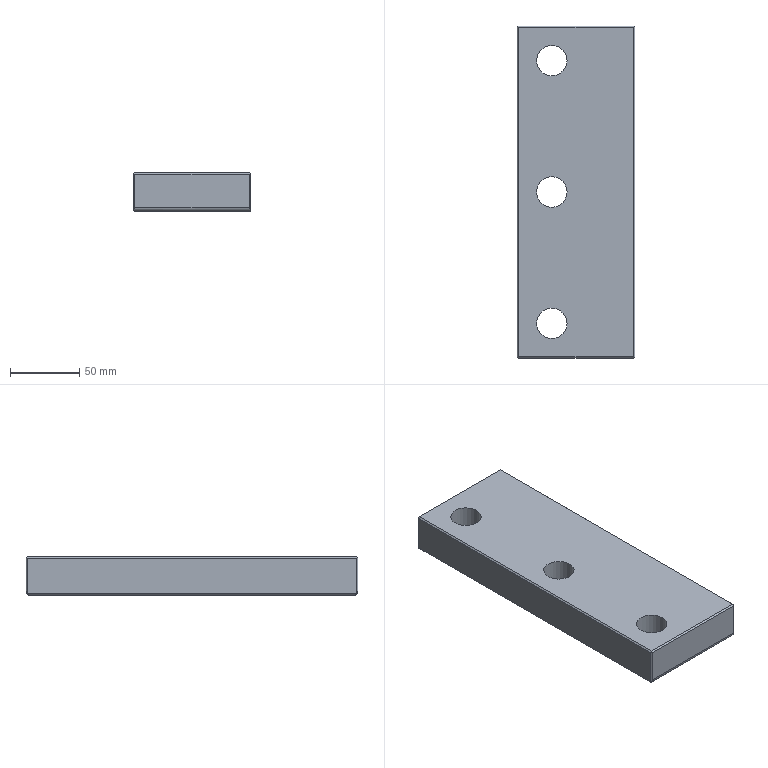Part | NX | features solid 2 | 1 solid | 21 faces | box 85 x 240 x 28 mm | volume 538397 mm3 | plane 15 | cylinder 6 | commonest cylinder face diameters 22 x3 6 x2 2 x1
STEP:
#1=CARTESIAN_POINT('',(-565.,441.,89.));
#2=VERTEX_POINT('',#1);
#3=CARTESIAN_POINT('',(-565.,441.,63.));
#4=VERTEX_POINT('',#3);
#5=CARTESIAN_POINT('',(-565.,441.,62.));
#6=DIRECTION('',(0.,0.,-1.));
#7=VECTOR('',#6,1000.);
#8=LINE('',#5,#7);
#9=EDGE_CURVE('',#2,#4,#8,.T.);
#10=ORIENTED_EDGE('',*,*,#9,.T.);
#11=CARTESIAN_POINT('',(-565.,679.,63.));
#12=VERTEX_POINT('',#11);
#13=CARTESIAN_POINT('',(-565.,680.,63.));
#14=DIRECTION('',(0.,-1.,0.));
#15=VECTOR('',#14,1000.);
#16=LINE('',#13,#15);
#17=EDGE_CURVE('',#4,#12,#16,.F.);
#18=ORIENTED_EDGE('',*,*,#17,.T.);
#19=CARTESIAN_POINT('',(-565.,679.,89.));
#20=VERTEX_POINT('',#19);
#21=CARTESIAN_POINT('',(-565.,679.,62.));
#22=DIRECTION('',(0.,0.,1.));
#23=VECTOR('',#22,1000.);
#24=LINE('',#21,#23);
#25=EDGE_CURVE('',#12,#20,#24,.T.);
#26=ORIENTED_EDGE('',*,*,#25,.T.);
#27=CARTESIAN_POINT('',(-565.,680.,89.));
#28=DIRECTION('',(0.,-1.,0.));
#29=VECTOR('',#28,1000.);
#30=LINE('',#27,#29);
#31=EDGE_CURVE('',#20,#2,#30,.T.);
#32=ORIENTED_EDGE('',*,*,#31,.T.);
#33=EDGE_LOOP('',(#10,#18,#26,#32));
#34=FACE_BOUND('',#33,.T.);
#35=CARTESIAN_POINT('',(-565.,680.,62.));
#36=DIRECTION('',(1.,0.,0.));
#37=DIRECTION('',(0.,0.,-1.));
#38=AXIS2_PLACEMENT_3D('',#35,#36,#37);
#39=PLANE('',#38);
#40=ADVANCED_FACE('',(#34),#39,.T.);
#41=CARTESIAN_POINT('',(-614.,655.,90.));
#42=VERTEX_POINT('',#41);
#43=CARTESIAN_POINT('',(-625.,655.,90.));
#44=DIRECTION('',(0.,0.,1.));
#45=DIRECTION('',(1.,0.,0.));
#46=AXIS2_PLACEMENT_3D('',#43,#44,#45);
#47=CIRCLE('',#46,11.);
#48=EDGE_CURVE('',#42,#42,#47,.T.);
#49=ORIENTED_EDGE('',*,*,#48,.F.);
#50=EDGE_LOOP('',(#49));
#51=FACE_BOUND('',#50,.T.);
#52=CARTESIAN_POINT('',(-614.,560.,90.));
#53=VERTEX_POINT('',#52);
#54=CARTESIAN_POINT('',(-625.,560.,90.));
#55=DIRECTION('',(0.,0.,1.));
#56=DIRECTION('',(1.,0.,0.));
#57=AXIS2_PLACEMENT_3D('',#54,#55,#56);
#58=CIRCLE('',#57,11.);
#59=EDGE_CURVE('',#53,#53,#58,.T.);
#60=ORIENTED_EDGE('',*,*,#59,.F.);
#61=EDGE_LOOP('',(#60));
#62=FACE_BOUND('',#61,.T.);
#63=CARTESIAN_POINT('',(-614.,465.,90.));
#64=VERTEX_POINT('',#63);
#65=CARTESIAN_POINT('',(-625.,465.,90.));
#66=DIRECTION('',(0.,0.,1.));
#67=DIRECTION('',(1.,0.,0.));
#68=AXIS2_PLACEMENT_3D('',#65,#66,#67);
#69=CIRCLE('',#68,11.);
#70=EDGE_CURVE('',#64,#64,#69,.T.);
#71=ORIENTED_EDGE('',*,*,#70,.F.);
#72=EDGE_LOOP('',(#71));
#73=FACE_BOUND('',#72,.T.);
#74=CARTESIAN_POINT('',(-649.,679.,90.));
#75=VERTEX_POINT('',#74);
#76=CARTESIAN_POINT('',(-649.,441.,90.));
#77=VERTEX_POINT('',#76);
#78=CARTESIAN_POINT('',(-649.,680.,90.));
#79=DIRECTION('',(0.,-1.,0.));
#80=VECTOR('',#79,1000.);
#81=LINE('',#78,#80);
#82=EDGE_CURVE('',#75,#77,#81,.T.);
#83=ORIENTED_EDGE('',*,*,#82,.T.);
#84=CARTESIAN_POINT('',(-566.,441.,90.));
#85=VERTEX_POINT('',#84);
#86=CARTESIAN_POINT('',(-566.,441.,90.));
#87=DIRECTION('',(1.,0.,0.));
#88=VECTOR('',#87,1000.);
#89=LINE('',#86,#88);
#90=EDGE_CURVE('',#77,#85,#89,.T.);
#91=ORIENTED_EDGE('',*,*,#90,.T.);
#92=CARTESIAN_POINT('',(-566.,679.,90.));
#93=VERTEX_POINT('',#92);
#94=CARTESIAN_POINT('',(-566.,680.,90.));
#95=DIRECTION('',(0.,1.,0.));
#96=VECTOR('',#95,1000.);
#97=LINE('',#94,#96);
#98=EDGE_CURVE('',#85,#93,#97,.T.);
#99=ORIENTED_EDGE('',*,*,#98,.T.);
#100=CARTESIAN_POINT('',(-565.,679.,90.));
#101=DIRECTION('',(-1.,0.,0.));
#102=VECTOR('',#101,1000.);
#103=LINE('',#100,#102);
#104=EDGE_CURVE('',#93,#75,#103,.T.);
#105=ORIENTED_EDGE('',*,*,#104,.T.);
#106=EDGE_LOOP('',(#83,#91,#99,#105));
#107=FACE_BOUND('',#106,.T.);
#108=CARTESIAN_POINT('',(-565.,680.,90.));
#109=DIRECTION('',(0.,0.,1.));
#110=DIRECTION('',(1.,0.,0.));
#111=AXIS2_PLACEMENT_3D('',#108,#109,#110);
#112=PLANE('',#111);
#113=ADVANCED_FACE('',(#51,#62,#73,#107),#112,.T.);
#114=CARTESIAN_POINT('',(-650.,441.,63.));
#115=VERTEX_POINT('',#114);
#116=CARTESIAN_POINT('',(-650.,441.,89.));
#117=VERTEX_POINT('',#116);
#118=CARTESIAN_POINT('',(-650.,441.,90.));
#119=DIRECTION('',(0.,0.,1.));
#120=VECTOR('',#119,1000.);
#121=LINE('',#118,#120);
#122=EDGE_CURVE('',#115,#117,#121,.T.);
#123=ORIENTED_EDGE('',*,*,#122,.T.);
#124=CARTESIAN_POINT('',(-650.,679.,89.));
#125=VERTEX_POINT('',#124);
#126=CARTESIAN_POINT('',(-650.,680.,89.));
#127=DIRECTION('',(0.,1.,0.));
#128=VECTOR('',#127,1000.);
#129=LINE('',#126,#128);
#130=EDGE_CURVE('',#117,#125,#129,.T.);
#131=ORIENTED_EDGE('',*,*,#130,.T.);
#132=CARTESIAN_POINT('',(-650.,679.,63.));
#133=VERTEX_POINT('',#132);
#134=CARTESIAN_POINT('',(-650.,679.,90.));
#135=DIRECTION('',(0.,0.,-1.));
#136=VECTOR('',#135,1000.);
#137=LINE('',#134,#136);
#138=EDGE_CURVE('',#125,#133,#137,.T.);
#139=ORIENTED_EDGE('',*,*,#138,.T.);
#140=CARTESIAN_POINT('',(-650.,680.,63.));
#141=DIRECTION('',(0.,-1.,0.));
#142=VECTOR('',#141,1000.);
#143=LINE('',#140,#142);
#144=EDGE_CURVE('',#133,#115,#143,.T.);
#145=ORIENTED_EDGE('',*,*,#144,.T.);
#146=EDGE_LOOP('',(#123,#131,#139,#145));
#147=FACE_BOUND('',#146,.T.);
#148=CARTESIAN_POINT('',(-650.,680.,90.));
#149=DIRECTION('',(-1.,0.,0.));
#150=DIRECTION('',(0.,0.,1.));
#151=AXIS2_PLACEMENT_3D('',#148,#149,#150);
#152=PLANE('',#151);
#153=ADVANCED_FACE('',(#147),#152,.T.);
#154=CARTESIAN_POINT('',(-614.,655.,62.));
#155=VERTEX_POINT('',#154);
#156=CARTESIAN_POINT('',(-625.,655.,62.));
#157=DIRECTION('',(0.,0.,1.));
#158=DIRECTION('',(1.,0.,0.));
#159=AXIS2_PLACEMENT_3D('',#156,#157,#158);
#160=CIRCLE('',#159,11.);
#161=EDGE_CURVE('',#155,#155,#160,.T.);
#162=ORIENTED_EDGE('',*,*,#161,.T.);
#163=EDGE_LOOP('',(#162));
#164=FACE_BOUND('',#163,.T.);
#165=CARTESIAN_POINT('',(-614.,560.,62.));
#166=VERTEX_POINT('',#165);
#167=CARTESIAN_POINT('',(-625.,560.,62.));
#168=DIRECTION('',(0.,0.,1.));
#169=DIRECTION('',(1.,0.,0.));
#170=AXIS2_PLACEMENT_3D('',#167,#168,#169);
#171=CIRCLE('',#170,11.);
#172=EDGE_CURVE('',#166,#166,#171,.T.);
#173=ORIENTED_EDGE('',*,*,#172,.T.);
#174=EDGE_LOOP('',(#173));
#175=FACE_BOUND('',#174,.T.);
#176=CARTESIAN_POINT('',(-614.,465.,62.));
#177=VERTEX_POINT('',#176);
#178=CARTESIAN_POINT('',(-625.,465.,62.));
#179=DIRECTION('',(0.,0.,1.));
#180=DIRECTION('',(1.,0.,0.));
#181=AXIS2_PLACEMENT_3D('',#178,#179,#180);
#182=CIRCLE('',#181,11.);
#183=EDGE_CURVE('',#177,#177,#182,.T.);
#184=ORIENTED_EDGE('',*,*,#183,.T.);
#185=EDGE_LOOP('',(#184));
#186=FACE_BOUND('',#185,.T.);
#187=CARTESIAN_POINT('',(-649.,443.,62.));
#188=VERTEX_POINT('',#187);
#189=CARTESIAN_POINT('',(-649.,677.,62.));
#190=VERTEX_POINT('',#189);
#191=CARTESIAN_POINT('',(-649.,680.,62.));
#192=DIRECTION('',(0.,1.,0.));
#193=VECTOR('',#192,1000.);
#194=LINE('',#191,#193);
#195=EDGE_CURVE('',#188,#190,#194,.T.);
#196=ORIENTED_EDGE('',*,*,#195,.T.);
#197=CARTESIAN_POINT('',(-566.,677.,62.));
#198=VERTEX_POINT('',#197);
#199=CARTESIAN_POINT('',(-650.,677.,62.));
#200=DIRECTION('',(1.,0.,0.));
#201=VECTOR('',#200,1000.);
#202=LINE('',#199,#201);
#203=EDGE_CURVE('',#190,#198,#202,.T.);
#204=ORIENTED_EDGE('',*,*,#203,.T.);
#205=CARTESIAN_POINT('',(-566.,443.,62.));
#206=VERTEX_POINT('',#205);
#207=CARTESIAN_POINT('',(-566.,680.,62.));
#208=DIRECTION('',(0.,-1.,0.));
#209=VECTOR('',#208,1000.);
#210=LINE('',#207,#209);
#211=EDGE_CURVE('',#198,#206,#210,.T.);
#212=ORIENTED_EDGE('',*,*,#211,.T.);
#213=CARTESIAN_POINT('',(-649.,443.,62.));
#214=DIRECTION('',(1.,0.,0.));
#215=VECTOR('',#214,1000.);
#216=LINE('',#213,#215);
#217=EDGE_CURVE('',#206,#188,#216,.F.);
#218=ORIENTED_EDGE('',*,*,#217,.T.);
#219=EDGE_LOOP('',(#196,#204,#212,#218));
#220=FACE_BOUND('',#219,.T.);
#221=CARTESIAN_POINT('',(-650.,680.,62.));
#222=DIRECTION('',(0.,0.,-1.));
#223=DIRECTION('',(-1.,0.,0.));
#224=AXIS2_PLACEMENT_3D('',#221,#222,#223);
#225=PLANE('',#224);
#226=ADVANCED_FACE('',(#164,#175,#186,#220),#225,.T.);
#227=CARTESIAN_POINT('',(-649.,680.,65.));
#228=VERTEX_POINT('',#227);
#229=CARTESIAN_POINT('',(-649.,680.,89.));
#230=VERTEX_POINT('',#229);
#231=CARTESIAN_POINT('',(-649.,680.,62.));
#232=DIRECTION('',(0.,0.,1.));
#233=VECTOR('',#232,1000.);
#234=LINE('',#231,#233);
#235=EDGE_CURVE('',#228,#230,#234,.T.);
#236=ORIENTED_EDGE('',*,*,#235,.T.);
#237=CARTESIAN_POINT('',(-566.,680.,89.));
#238=VERTEX_POINT('',#237);
#239=CARTESIAN_POINT('',(-565.,680.,89.));
#240=DIRECTION('',(1.,0.,0.));
#241=VECTOR('',#240,1000.);
#242=LINE('',#239,#241);
#243=EDGE_CURVE('',#230,#238,#242,.T.);
#244=ORIENTED_EDGE('',*,*,#243,.T.);
#245=CARTESIAN_POINT('',(-566.,680.,65.));
#246=VERTEX_POINT('',#245);
#247=CARTESIAN_POINT('',(-566.,680.,62.));
#248=DIRECTION('',(0.,0.,-1.));
#249=VECTOR('',#248,1000.);
#250=LINE('',#247,#249);
#251=EDGE_CURVE('',#238,#246,#250,.T.);
#252=ORIENTED_EDGE('',*,*,#251,.T.);
#253=CARTESIAN_POINT('',(-565.,680.,65.));
#254=DIRECTION('',(1.,0.,0.));
#255=VECTOR('',#254,1000.);
#256=LINE('',#253,#255);
#257=EDGE_CURVE('',#246,#228,#256,.F.);
#258=ORIENTED_EDGE('',*,*,#257,.T.);
#259=EDGE_LOOP('',(#236,#244,#252,#258));
#260=FACE_BOUND('',#259,.T.);
#261=CARTESIAN_POINT('',(-565.,680.,62.));
#262=DIRECTION('',(0.,1.,0.));
#263=DIRECTION('',(0.,0.,1.));
#264=AXIS2_PLACEMENT_3D('',#261,#262,#263);
#265=PLANE('',#264);
#266=ADVANCED_FACE('',(#260),#265,.T.);
#267=CARTESIAN_POINT('',(-566.,440.,65.));
#268=VERTEX_POINT('',#267);
#269=CARTESIAN_POINT('',(-566.,440.,89.));
#270=VERTEX_POINT('',#269);
#271=CARTESIAN_POINT('',(-566.,440.,90.));
#272=DIRECTION('',(0.,0.,1.));
#273=VECTOR('',#272,1000.);
#274=LINE('',#271,#273);
#275=EDGE_CURVE('',#268,#270,#274,.T.);
#276=ORIENTED_EDGE('',*,*,#275,.T.);
#277=CARTESIAN_POINT('',(-649.,440.,89.));
#278=VERTEX_POINT('',#277);
#279=CARTESIAN_POINT('',(-649.,440.,89.));
#280=DIRECTION('',(-1.,0.,0.));
#281=VECTOR('',#280,1000.);
#282=LINE('',#279,#281);
#283=EDGE_CURVE('',#270,#278,#282,.T.);
#284=ORIENTED_EDGE('',*,*,#283,.T.);
#285=CARTESIAN_POINT('',(-649.,440.,65.));
#286=VERTEX_POINT('',#285);
#287=CARTESIAN_POINT('',(-649.,440.,62.));
#288=DIRECTION('',(0.,0.,-1.));
#289=VECTOR('',#288,1000.);
#290=LINE('',#287,#289);
#291=EDGE_CURVE('',#278,#286,#290,.T.);
#292=ORIENTED_EDGE('',*,*,#291,.T.);
#293=CARTESIAN_POINT('',(-566.,440.,65.));
#294=DIRECTION('',(1.,0.,0.));
#295=VECTOR('',#294,1000.);
#296=LINE('',#293,#295);
#297=EDGE_CURVE('',#286,#268,#296,.T.);
#298=ORIENTED_EDGE('',*,*,#297,.T.);
#299=EDGE_LOOP('',(#276,#284,#292,#298));
#300=FACE_BOUND('',#299,.T.);
#301=CARTESIAN_POINT('',(-565.,440.,62.));
#302=DIRECTION('',(0.,1.,0.));
#303=DIRECTION('',(0.,0.,1.));
#304=AXIS2_PLACEMENT_3D('',#301,#302,#303);
#305=PLANE('',#304);
#306=ADVANCED_FACE('',(#300),#305,.F.);
#307=ORIENTED_EDGE('',*,*,#70,.T.);
#308=EDGE_LOOP('',(#307));
#309=FACE_BOUND('',#308,.T.);
#310=ORIENTED_EDGE('',*,*,#183,.F.);
#311=EDGE_LOOP('',(#310));
#312=FACE_BOUND('',#311,.T.);
#313=CARTESIAN_POINT('',(-625.,465.,62.));
#314=DIRECTION('',(0.,0.,1.));
#315=DIRECTION('',(1.,0.,0.));
#316=AXIS2_PLACEMENT_3D('',#313,#314,#315);
#317=CYLINDRICAL_SURFACE('',#316,11.);
#318=ADVANCED_FACE('',(#309,#312),#317,.F.);
#319=ORIENTED_EDGE('',*,*,#251,.F.);
#320=CARTESIAN_POINT('',(-565.5,679.5,89.5));
#321=VERTEX_POINT('',#320);
#322=CARTESIAN_POINT('',(-574.333,688.333,80.667));
#323=DIRECTION('',(0.5774,-0.5774,0.5774));
#324=VECTOR('',#323,1000.);
#325=LINE('',#322,#324);
#326=EDGE_CURVE('',#238,#321,#325,.T.);
#327=ORIENTED_EDGE('',*,*,#326,.T.);
#328=CARTESIAN_POINT('',(-556.,670.,80.));
#329=DIRECTION('',(0.5774,-0.5774,-0.5774));
#330=VECTOR('',#329,1000.);
#331=LINE('',#328,#330);
#332=EDGE_CURVE('',#321,#20,#331,.T.);
#333=ORIENTED_EDGE('',*,*,#332,.T.);
#334=ORIENTED_EDGE('',*,*,#25,.F.);
#335=CARTESIAN_POINT('',(-565.023,679.023,62.785));
#336=VERTEX_POINT('',#335);
#337=CARTESIAN_POINT('',(-566.,680.,63.));
#338=DIRECTION('',(-0.7071,-0.7071,0.));
#339=DIRECTION('',(0.7071,-0.7071,0.));
#340=AXIS2_PLACEMENT_3D('',#337,#338,#339);
#341=ELLIPSE('',#340,1.414,1.);
#342=EDGE_CURVE('',#12,#336,#341,.F.);
#343=ORIENTED_EDGE('',*,*,#342,.T.);
#344=CARTESIAN_POINT('',(-563.,677.,65.));
#345=DIRECTION('',(-0.7071,-0.7071,0.));
#346=DIRECTION('',(0.7071,-0.7071,0.));
#347=AXIS2_PLACEMENT_3D('',#344,#345,#346);
#348=ELLIPSE('',#347,4.243,3.);
#349=EDGE_CURVE('',#336,#246,#348,.F.);
#350=ORIENTED_EDGE('',*,*,#349,.T.);
#351=EDGE_LOOP('',(#319,#327,#333,#334,#343,#350));
#352=FACE_BOUND('',#351,.T.);
#353=CARTESIAN_POINT('',(-565.,679.,62.));
#354=DIRECTION('',(-0.7071,-0.7071,0.));
#355=DIRECTION('',(-0.7071,0.7071,0.));
#356=AXIS2_PLACEMENT_3D('',#353,#354,#355);
#357=PLANE('',#356);
#358=ADVANCED_FACE('',(#352),#357,.F.);
#359=CARTESIAN_POINT('',(-649.5,679.5,89.5));
#360=VERTEX_POINT('',#359);
#361=CARTESIAN_POINT('',(-649.667,679.333,89.333));
#362=DIRECTION('',(0.5774,0.5774,0.5774));
#363=VECTOR('',#362,1000.);
#364=LINE('',#361,#363);
#365=EDGE_CURVE('',#125,#360,#364,.T.);
#366=ORIENTED_EDGE('',*,*,#365,.T.);
#367=CARTESIAN_POINT('',(-650.,679.,90.));
#368=DIRECTION('',(0.5774,0.5774,-0.5774));
#369=VECTOR('',#368,1000.);
#370=LINE('',#367,#369);
#371=EDGE_CURVE('',#360,#230,#370,.T.);
#372=ORIENTED_EDGE('',*,*,#371,.T.);
#373=ORIENTED_EDGE('',*,*,#235,.F.);
#374=CARTESIAN_POINT('',(-649.879,679.121,62.879));
#375=VERTEX_POINT('',#374);
#376=CARTESIAN_POINT('',(-652.,677.,65.));
#377=DIRECTION('',(0.7071,-0.7071,0.));
#378=DIRECTION('',(0.7071,0.7071,0.));
#379=AXIS2_PLACEMENT_3D('',#376,#377,#378);
#380=ELLIPSE('',#379,4.243,3.);
#381=EDGE_CURVE('',#228,#375,#380,.F.);
#382=ORIENTED_EDGE('',*,*,#381,.T.);
#383=CARTESIAN_POINT('',(-659.,670.,72.));
#384=DIRECTION('',(-0.5774,-0.5774,0.5774));
#385=VECTOR('',#384,1000.);
#386=LINE('',#383,#385);
#387=EDGE_CURVE('',#375,#133,#386,.T.);
#388=ORIENTED_EDGE('',*,*,#387,.T.);
#389=ORIENTED_EDGE('',*,*,#138,.F.);
#390=EDGE_LOOP('',(#366,#372,#373,#382,#388,#389));
#391=FACE_BOUND('',#390,.T.);
#392=CARTESIAN_POINT('',(-650.,679.,90.));
#393=DIRECTION('',(0.7071,-0.7071,0.));
#394=DIRECTION('',(-0.7071,-0.7071,0.));
#395=AXIS2_PLACEMENT_3D('',#392,#393,#394);
#396=PLANE('',#395);
#397=ADVANCED_FACE('',(#391),#396,.F.);
#398=CARTESIAN_POINT('',(-565.023,440.977,62.785));
#399=VERTEX_POINT('',#398);
#400=CARTESIAN_POINT('',(-563.,443.,65.));
#401=DIRECTION('',(0.7071,-0.7071,0.));
#402=DIRECTION('',(-0.7071,-0.7071,0.));
#403=AXIS2_PLACEMENT_3D('',#400,#401,#402);
#404=ELLIPSE('',#403,4.243,3.);
#405=EDGE_CURVE('',#268,#399,#404,.T.);
#406=ORIENTED_EDGE('',*,*,#405,.T.);
#407=CARTESIAN_POINT('',(-566.,440.,63.));
#408=DIRECTION('',(0.7071,-0.7071,0.));
#409=DIRECTION('',(-0.7071,-0.7071,0.));
#410=AXIS2_PLACEMENT_3D('',#407,#408,#409);
#411=ELLIPSE('',#410,1.414,1.);
#412=EDGE_CURVE('',#399,#4,#411,.T.);
#413=ORIENTED_EDGE('',*,*,#412,.T.);
#414=ORIENTED_EDGE('',*,*,#9,.F.);
#415=CARTESIAN_POINT('',(-565.5,440.5,89.5));
#416=VERTEX_POINT('',#415);
#417=CARTESIAN_POINT('',(-556.667,449.333,80.667));
#418=DIRECTION('',(0.5774,0.5774,-0.5774));
#419=VECTOR('',#418,1000.);
#420=LINE('',#417,#419);
#421=EDGE_CURVE('',#2,#416,#420,.F.);
#422=ORIENTED_EDGE('',*,*,#421,.T.);
#423=CARTESIAN_POINT('',(-575.,431.,80.));
#424=DIRECTION('',(-0.5774,-0.5774,-0.5774));
#425=VECTOR('',#424,1000.);
#426=LINE('',#423,#425);
#427=EDGE_CURVE('',#416,#270,#426,.T.);
#428=ORIENTED_EDGE('',*,*,#427,.T.);
#429=ORIENTED_EDGE('',*,*,#275,.F.);
#430=EDGE_LOOP('',(#406,#413,#414,#422,#428,#429));
#431=FACE_BOUND('',#430,.T.);
#432=CARTESIAN_POINT('',(-566.,440.,62.));
#433=DIRECTION('',(0.7071,-0.7071,0.));
#434=DIRECTION('',(-0.7071,-0.7071,0.));
#435=AXIS2_PLACEMENT_3D('',#432,#433,#434);
#436=PLANE('',#435);
#437=ADVANCED_FACE('',(#431),#436,.T.);
#438=ORIENTED_EDGE('',*,*,#291,.F.);
#439=CARTESIAN_POINT('',(-649.5,440.5,89.5));
#440=VERTEX_POINT('',#439);
#441=CARTESIAN_POINT('',(-640.,431.,80.));
#442=DIRECTION('',(-0.5774,0.5774,0.5774));
#443=VECTOR('',#442,1000.);
#444=LINE('',#441,#443);
#445=EDGE_CURVE('',#278,#440,#444,.T.);
#446=ORIENTED_EDGE('',*,*,#445,.T.);
#447=CARTESIAN_POINT('',(-658.333,449.333,80.667));
#448=DIRECTION('',(0.5774,-0.5774,0.5774));
#449=VECTOR('',#448,1000.);
#450=LINE('',#447,#449);
#451=EDGE_CURVE('',#440,#117,#450,.F.);
#452=ORIENTED_EDGE('',*,*,#451,.T.);
#453=ORIENTED_EDGE('',*,*,#122,.F.);
#454=CARTESIAN_POINT('',(-649.879,440.879,62.879));
#455=VERTEX_POINT('',#454);
#456=CARTESIAN_POINT('',(-649.,440.,62.));
#457=DIRECTION('',(-0.5774,0.5774,0.5774));
#458=VECTOR('',#457,1000.);
#459=LINE('',#456,#458);
#460=EDGE_CURVE('',#115,#455,#459,.F.);
#461=ORIENTED_EDGE('',*,*,#460,.T.);
#462=CARTESIAN_POINT('',(-652.,443.,65.));
#463=DIRECTION('',(-0.7071,-0.7071,0.));
#464=DIRECTION('',(-0.7071,0.7071,0.));
#465=AXIS2_PLACEMENT_3D('',#462,#463,#464);
#466=ELLIPSE('',#465,4.243,3.);
#467=EDGE_CURVE('',#455,#286,#466,.T.);
#468=ORIENTED_EDGE('',*,*,#467,.T.);
#469=EDGE_LOOP('',(#438,#446,#452,#453,#461,#468));
#470=FACE_BOUND('',#469,.T.);
#471=CARTESIAN_POINT('',(-649.,440.,62.));
#472=DIRECTION('',(-0.7071,-0.7071,0.));
#473=DIRECTION('',(-0.7071,0.7071,0.));
#474=AXIS2_PLACEMENT_3D('',#471,#472,#473);
#475=PLANE('',#474);
#476=ADVANCED_FACE('',(#470),#475,.T.);
#477=ORIENTED_EDGE('',*,*,#98,.F.);
#478=CARTESIAN_POINT('',(-631.667,506.667,155.667));
#479=DIRECTION('',(-0.5774,0.5774,0.5774));
#480=VECTOR('',#479,1000.);
#481=LINE('',#478,#480);
#482=EDGE_CURVE('',#85,#416,#481,.F.);
#483=ORIENTED_EDGE('',*,*,#482,.T.);
#484=ORIENTED_EDGE('',*,*,#421,.F.);
#485=ORIENTED_EDGE('',*,*,#31,.F.);
#486=ORIENTED_EDGE('',*,*,#332,.F.);
#487=CARTESIAN_POINT('',(-565.,680.,89.));
#488=DIRECTION('',(-0.5774,-0.5774,0.5774));
#489=VECTOR('',#488,1000.);
#490=LINE('',#487,#489);
#491=EDGE_CURVE('',#321,#93,#490,.T.);
#492=ORIENTED_EDGE('',*,*,#491,.T.);
#493=EDGE_LOOP('',(#477,#483,#484,#485,#486,#492));
#494=FACE_BOUND('',#493,.T.);
#495=CARTESIAN_POINT('',(-565.,680.,89.));
#496=DIRECTION('',(-0.7071,0.,-0.7071));
#497=DIRECTION('',(-0.7071,0.,0.7071));
#498=AXIS2_PLACEMENT_3D('',#495,#496,#497);
#499=PLANE('',#498);
#500=ADVANCED_FACE('',(#494),#499,.F.);
#501=ORIENTED_EDGE('',*,*,#451,.F.);
#502=CARTESIAN_POINT('',(-582.667,507.333,156.333));
#503=DIRECTION('',(-0.5774,-0.5774,-0.5774));
#504=VECTOR('',#503,1000.);
#505=LINE('',#502,#504);
#506=EDGE_CURVE('',#440,#77,#505,.F.);
#507=ORIENTED_EDGE('',*,*,#506,.T.);
#508=ORIENTED_EDGE('',*,*,#82,.F.);
#509=CARTESIAN_POINT('',(-649.333,679.333,89.667));
#510=DIRECTION('',(-0.5774,0.5774,-0.5774));
#511=VECTOR('',#510,1000.);
#512=LINE('',#509,#511);
#513=EDGE_CURVE('',#75,#360,#512,.T.);
#514=ORIENTED_EDGE('',*,*,#513,.T.);
#515=ORIENTED_EDGE('',*,*,#365,.F.);
#516=ORIENTED_EDGE('',*,*,#130,.F.);
#517=EDGE_LOOP('',(#501,#507,#508,#514,#515,#516));
#518=FACE_BOUND('',#517,.T.);
#519=CARTESIAN_POINT('',(-649.,680.,90.));
#520=DIRECTION('',(0.7071,0.,-0.7071));
#521=DIRECTION('',(-0.7071,0.,-0.7071));
#522=AXIS2_PLACEMENT_3D('',#519,#520,#521);
#523=PLANE('',#522);
#524=ADVANCED_FACE('',(#518),#523,.F.);
#525=ORIENTED_EDGE('',*,*,#387,.F.);
#526=CARTESIAN_POINT('',(-652.,677.,65.));
#527=DIRECTION('',(0.7071,0.,0.7071));
#528=DIRECTION('',(0.7071,0.,-0.7071));
#529=AXIS2_PLACEMENT_3D('',#526,#527,#528);
#530=ELLIPSE('',#529,4.243,3.);
#531=EDGE_CURVE('',#375,#190,#530,.F.);
#532=ORIENTED_EDGE('',*,*,#531,.T.);
#533=ORIENTED_EDGE('',*,*,#195,.F.);
#534=CARTESIAN_POINT('',(-652.,443.,65.));
#535=DIRECTION('',(0.7071,0.,0.7071));
#536=DIRECTION('',(-0.7071,0.,0.7071));
#537=AXIS2_PLACEMENT_3D('',#534,#535,#536);
#538=ELLIPSE('',#537,4.243,3.);
#539=EDGE_CURVE('',#188,#455,#538,.F.);
#540=ORIENTED_EDGE('',*,*,#539,.T.);
#541=ORIENTED_EDGE('',*,*,#460,.F.);
#542=ORIENTED_EDGE('',*,*,#144,.F.);
#543=EDGE_LOOP('',(#525,#532,#533,#540,#541,#542));
#544=FACE_BOUND('',#543,.T.);
#545=CARTESIAN_POINT('',(-650.,680.,63.));
#546=DIRECTION('',(0.7071,0.,0.7071));
#547=DIRECTION('',(0.7071,0.,-0.7071));
#548=AXIS2_PLACEMENT_3D('',#545,#546,#547);
#549=PLANE('',#548);
#550=ADVANCED_FACE('',(#544),#549,.F.);
#551=ORIENTED_EDGE('',*,*,#211,.F.);
#552=CARTESIAN_POINT('',(-565.023,679.023,62.785));
#553=CARTESIAN_POINT('',(-565.144,678.423,62.236));
#554=CARTESIAN_POINT('',(-565.595,677.702,62.));
#555=CARTESIAN_POINT('',(-566.,677.,62.));
#556=B_SPLINE_CURVE_WITH_KNOTS('',3,(#552,#553,#554,#555),.UNSPECIFIED.,.F.,.F.,(4,4),(0.,0.002432),.UNSPECIFIED.);
#557=EDGE_CURVE('',#198,#336,#556,.F.);
#558=ORIENTED_EDGE('',*,*,#557,.T.);
#559=ORIENTED_EDGE('',*,*,#342,.F.);
#560=ORIENTED_EDGE('',*,*,#17,.F.);
#561=ORIENTED_EDGE('',*,*,#412,.F.);
#562=CARTESIAN_POINT('',(-565.023,440.977,62.785));
#563=CARTESIAN_POINT('',(-565.144,441.576,62.237));
#564=CARTESIAN_POINT('',(-565.592,442.294,62.));
#565=CARTESIAN_POINT('',(-566.,443.,62.));
#566=B_SPLINE_CURVE_WITH_KNOTS('',3,(#562,#563,#564,#565),.UNSPECIFIED.,.F.,.F.,(4,4),(0.001838,0.004284),.UNSPECIFIED.);
#567=EDGE_CURVE('',#399,#206,#566,.T.);
#568=ORIENTED_EDGE('',*,*,#567,.T.);
#569=EDGE_LOOP('',(#551,#558,#559,#560,#561,#568));
#570=FACE_BOUND('',#569,.T.);
#571=CARTESIAN_POINT('',(-566.,680.,63.));
#572=DIRECTION('',(0.,-1.,0.));
#573=DIRECTION('',(0.,0.,-1.));
#574=AXIS2_PLACEMENT_3D('',#571,#572,#573);
#575=CYLINDRICAL_SURFACE('',#574,1.);
#576=ADVANCED_FACE('',(#570),#575,.T.);
#577=ORIENTED_EDGE('',*,*,#59,.T.);
#578=EDGE_LOOP('',(#577));
#579=FACE_BOUND('',#578,.T.);
#580=ORIENTED_EDGE('',*,*,#172,.F.);
#581=EDGE_LOOP('',(#580));
#582=FACE_BOUND('',#581,.T.);
#583=CARTESIAN_POINT('',(-625.,560.,62.));
#584=DIRECTION('',(0.,0.,1.));
#585=DIRECTION('',(1.,0.,0.));
#586=AXIS2_PLACEMENT_3D('',#583,#584,#585);
#587=CYLINDRICAL_SURFACE('',#586,11.);
#588=ADVANCED_FACE('',(#579,#582),#587,.F.);
#589=ORIENTED_EDGE('',*,*,#48,.T.);
#590=EDGE_LOOP('',(#589));
#591=FACE_BOUND('',#590,.T.);
#592=ORIENTED_EDGE('',*,*,#161,.F.);
#593=EDGE_LOOP('',(#592));
#594=FACE_BOUND('',#593,.T.);
#595=CARTESIAN_POINT('',(-625.,655.,62.));
#596=DIRECTION('',(0.,0.,1.));
#597=DIRECTION('',(1.,0.,0.));
#598=AXIS2_PLACEMENT_3D('',#595,#596,#597);
#599=CYLINDRICAL_SURFACE('',#598,11.);
#600=ADVANCED_FACE('',(#591,#594),#599,.F.);
#601=ORIENTED_EDGE('',*,*,#381,.F.);
#602=ORIENTED_EDGE('',*,*,#257,.F.);
#603=ORIENTED_EDGE('',*,*,#349,.F.);
#604=ORIENTED_EDGE('',*,*,#557,.F.);
#605=ORIENTED_EDGE('',*,*,#203,.F.);
#606=ORIENTED_EDGE('',*,*,#531,.F.);
#607=EDGE_LOOP('',(#601,#602,#603,#604,#605,#606));
#608=FACE_BOUND('',#607,.T.);
#609=CARTESIAN_POINT('',(-650.,677.,65.));
#610=DIRECTION('',(1.,0.,0.));
#611=DIRECTION('',(0.,0.,-1.));
#612=AXIS2_PLACEMENT_3D('',#609,#610,#611);
#613=CYLINDRICAL_SURFACE('',#612,3.);
#614=ADVANCED_FACE('',(#608),#613,.T.);
#615=ORIENTED_EDGE('',*,*,#567,.F.);
#616=ORIENTED_EDGE('',*,*,#405,.F.);
#617=ORIENTED_EDGE('',*,*,#297,.F.);
#618=ORIENTED_EDGE('',*,*,#467,.F.);
#619=ORIENTED_EDGE('',*,*,#539,.F.);
#620=ORIENTED_EDGE('',*,*,#217,.F.);
#621=EDGE_LOOP('',(#615,#616,#617,#618,#619,#620));
#622=FACE_BOUND('',#621,.T.);
#623=CARTESIAN_POINT('',(-565.,443.,65.));
#624=DIRECTION('',(-1.,0.,0.));
#625=DIRECTION('',(0.,0.,1.));
#626=AXIS2_PLACEMENT_3D('',#623,#624,#625);
#627=CYLINDRICAL_SURFACE('',#626,3.);
#628=ADVANCED_FACE('',(#622),#627,.T.);
#629=ORIENTED_EDGE('',*,*,#482,.F.);
#630=ORIENTED_EDGE('',*,*,#90,.F.);
#631=ORIENTED_EDGE('',*,*,#506,.F.);
#632=ORIENTED_EDGE('',*,*,#445,.F.);
#633=ORIENTED_EDGE('',*,*,#283,.F.);
#634=ORIENTED_EDGE('',*,*,#427,.F.);
#635=EDGE_LOOP('',(#629,#630,#631,#632,#633,#634));
#636=FACE_BOUND('',#635,.T.);
#637=CARTESIAN_POINT('',(-565.,440.,89.));
#638=DIRECTION('',(0.,-0.7071,0.7071));
#639=DIRECTION('',(0.,-0.7071,-0.7071));
#640=AXIS2_PLACEMENT_3D('',#637,#638,#639);
#641=PLANE('',#640);
#642=ADVANCED_FACE('',(#636),#641,.T.);
#643=ORIENTED_EDGE('',*,*,#326,.F.);
#644=ORIENTED_EDGE('',*,*,#243,.F.);
#645=ORIENTED_EDGE('',*,*,#371,.F.);
#646=ORIENTED_EDGE('',*,*,#513,.F.);
#647=ORIENTED_EDGE('',*,*,#104,.F.);
#648=ORIENTED_EDGE('',*,*,#491,.F.);
#649=EDGE_LOOP('',(#643,#644,#645,#646,#647,#648));
#650=FACE_BOUND('',#649,.T.);
#651=CARTESIAN_POINT('',(-565.,679.,90.));
#652=DIRECTION('',(0.,-0.7071,-0.7071));
#653=DIRECTION('',(0.,0.7071,-0.7071));
#654=AXIS2_PLACEMENT_3D('',#651,#652,#653);
#655=PLANE('',#654);
#656=ADVANCED_FACE('',(#650),#655,.F.);
#657=CLOSED_SHELL('',(#40,#113,#153,#226,#266,#306,#318,#358,#397,#437,#476,#500,#524,#550,#576,#588,#600,#614,#628,#642,#656));
#658=MANIFOLD_SOLID_BREP('',#657);
#659=(LENGTH_UNIT()NAMED_UNIT(*)SI_UNIT(.MILLI.,.METRE.));
#660=UNCERTAINTY_MEASURE_WITH_UNIT(LENGTH_MEASURE(0.0508),#659,'','');
#661=(NAMED_UNIT(*)PLANE_ANGLE_UNIT()SI_UNIT($,.RADIAN.));
#662=(NAMED_UNIT(*)SI_UNIT($,.STERADIAN.)SOLID_ANGLE_UNIT());
#663=(GEOMETRIC_REPRESENTATION_CONTEXT(3)GLOBAL_UNCERTAINTY_ASSIGNED_CONTEXT((#660))GLOBAL_UNIT_ASSIGNED_CONTEXT((#659,#661,#662))REPRESENTATION_CONTEXT('',''));
#664=ADVANCED_BREP_SHAPE_REPRESENTATION('',(#658),#663);